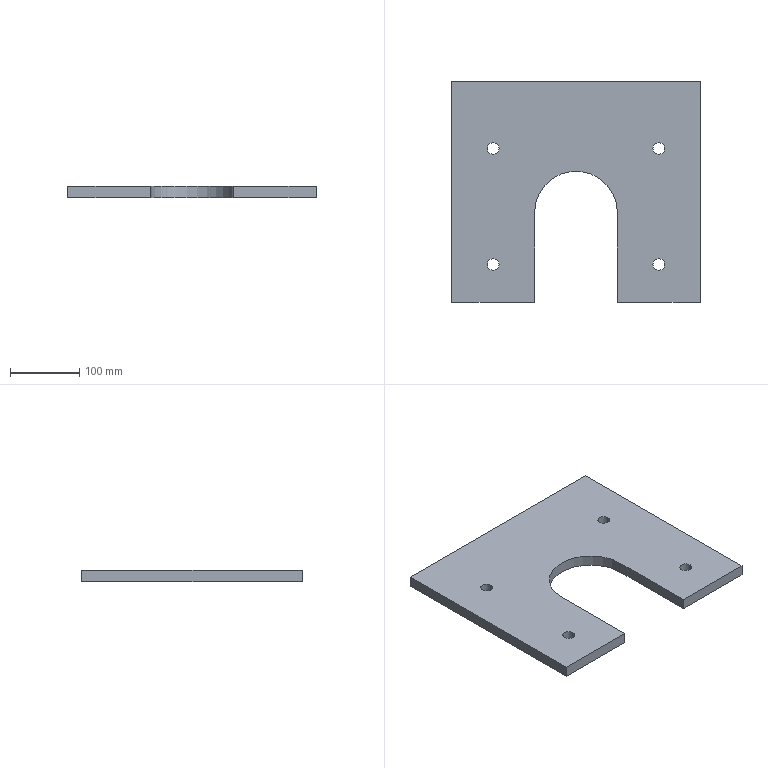Part | SolidWorks | features ICE 2, Extrusion 1, LPattern 1 | 1 solid | 18 faces | box 360 x 320 x 16 mm | volume 1488595 mm3 | cylinder 9 | plane 9 | commonest cylinder face diameters 17 x8 120 x1
STEP:
#1=CARTESIAN_POINT('',(111.5,-105.,-8.));
#2=VERTEX_POINT('',#1);
#3=CARTESIAN_POINT('',(128.5,-105.,-8.));
#4=VERTEX_POINT('',#3);
#5=CARTESIAN_POINT('',(120.,-105.,-8.));
#6=DIRECTION('',(0.,0.,1.));
#7=DIRECTION('',(1.,0.,0.));
#8=AXIS2_PLACEMENT_3D('',#5,#6,#7);
#9=CIRCLE('',#8,8.5);
#10=EDGE_CURVE('',#2,#4,#9,.T.);
#11=ORIENTED_EDGE('',*,*,#10,.F.);
#12=CARTESIAN_POINT('',(111.5,-105.,8.));
#13=VERTEX_POINT('',#12);
#14=CARTESIAN_POINT('',(111.5,-105.,-8.));
#15=DIRECTION('',(0.,0.,1.));
#16=VECTOR('',#15,1000.);
#17=LINE('',#14,#16);
#18=EDGE_CURVE('',#2,#13,#17,.T.);
#19=ORIENTED_EDGE('',*,*,#18,.T.);
#20=CARTESIAN_POINT('',(128.5,-105.,8.));
#21=VERTEX_POINT('',#20);
#22=CARTESIAN_POINT('',(120.,-105.,8.));
#23=DIRECTION('',(0.,0.,1.));
#24=DIRECTION('',(1.,0.,0.));
#25=AXIS2_PLACEMENT_3D('',#22,#23,#24);
#26=CIRCLE('',#25,8.5);
#27=EDGE_CURVE('',#13,#21,#26,.T.);
#28=ORIENTED_EDGE('',*,*,#27,.T.);
#29=CARTESIAN_POINT('',(128.5,-105.,-8.));
#30=DIRECTION('',(0.,0.,1.));
#31=VECTOR('',#30,1000.);
#32=LINE('',#29,#31);
#33=EDGE_CURVE('',#4,#21,#32,.T.);
#34=ORIENTED_EDGE('',*,*,#33,.F.);
#35=EDGE_LOOP('',(#11,#19,#28,#34));
#36=FACE_OUTER_BOUND('',#35,.T.);
#37=CARTESIAN_POINT('',(120.,-105.,-8.));
#38=DIRECTION('',(0.,0.,1.));
#39=DIRECTION('',(1.,0.,0.));
#40=AXIS2_PLACEMENT_3D('',#37,#38,#39);
#41=CYLINDRICAL_SURFACE('',#40,8.5);
#42=ADVANCED_FACE('',(#36),#41,.F.);
#43=CARTESIAN_POINT('',(-128.5,-105.,-8.));
#44=VERTEX_POINT('',#43);
#45=CARTESIAN_POINT('',(-111.5,-105.,-8.));
#46=VERTEX_POINT('',#45);
#47=CARTESIAN_POINT('',(-120.,-105.,-8.));
#48=DIRECTION('',(0.,0.,1.));
#49=DIRECTION('',(1.,0.,0.));
#50=AXIS2_PLACEMENT_3D('',#47,#48,#49);
#51=CIRCLE('',#50,8.5);
#52=EDGE_CURVE('',#44,#46,#51,.T.);
#53=ORIENTED_EDGE('',*,*,#52,.F.);
#54=CARTESIAN_POINT('',(-128.5,-105.,8.));
#55=VERTEX_POINT('',#54);
#56=CARTESIAN_POINT('',(-128.5,-105.,-8.));
#57=DIRECTION('',(0.,0.,1.));
#58=VECTOR('',#57,1000.);
#59=LINE('',#56,#58);
#60=EDGE_CURVE('',#44,#55,#59,.T.);
#61=ORIENTED_EDGE('',*,*,#60,.T.);
#62=CARTESIAN_POINT('',(-111.5,-105.,8.));
#63=VERTEX_POINT('',#62);
#64=CARTESIAN_POINT('',(-120.,-105.,8.));
#65=DIRECTION('',(0.,0.,1.));
#66=DIRECTION('',(1.,0.,0.));
#67=AXIS2_PLACEMENT_3D('',#64,#65,#66);
#68=CIRCLE('',#67,8.5);
#69=EDGE_CURVE('',#55,#63,#68,.T.);
#70=ORIENTED_EDGE('',*,*,#69,.T.);
#71=CARTESIAN_POINT('',(-111.5,-105.,-8.));
#72=DIRECTION('',(0.,0.,1.));
#73=VECTOR('',#72,1000.);
#74=LINE('',#71,#73);
#75=EDGE_CURVE('',#46,#63,#74,.T.);
#76=ORIENTED_EDGE('',*,*,#75,.F.);
#77=EDGE_LOOP('',(#53,#61,#70,#76));
#78=FACE_OUTER_BOUND('',#77,.T.);
#79=CARTESIAN_POINT('',(-120.,-105.,-8.));
#80=DIRECTION('',(0.,0.,1.));
#81=DIRECTION('',(1.,0.,0.));
#82=AXIS2_PLACEMENT_3D('',#79,#80,#81);
#83=CYLINDRICAL_SURFACE('',#82,8.5);
#84=ADVANCED_FACE('',(#78),#83,.F.);
#85=CARTESIAN_POINT('',(111.5,63.,-8.));
#86=VERTEX_POINT('',#85);
#87=CARTESIAN_POINT('',(128.5,63.,-8.));
#88=VERTEX_POINT('',#87);
#89=CARTESIAN_POINT('',(120.,63.,-8.));
#90=DIRECTION('',(0.,0.,1.));
#91=DIRECTION('',(1.,0.,0.));
#92=AXIS2_PLACEMENT_3D('',#89,#90,#91);
#93=CIRCLE('',#92,8.5);
#94=EDGE_CURVE('',#86,#88,#93,.T.);
#95=ORIENTED_EDGE('',*,*,#94,.F.);
#96=CARTESIAN_POINT('',(111.5,63.,8.));
#97=VERTEX_POINT('',#96);
#98=CARTESIAN_POINT('',(111.5,63.,-8.));
#99=DIRECTION('',(0.,0.,1.));
#100=VECTOR('',#99,1000.);
#101=LINE('',#98,#100);
#102=EDGE_CURVE('',#86,#97,#101,.T.);
#103=ORIENTED_EDGE('',*,*,#102,.T.);
#104=CARTESIAN_POINT('',(128.5,63.,8.));
#105=VERTEX_POINT('',#104);
#106=CARTESIAN_POINT('',(120.,63.,8.));
#107=DIRECTION('',(0.,0.,1.));
#108=DIRECTION('',(1.,0.,0.));
#109=AXIS2_PLACEMENT_3D('',#106,#107,#108);
#110=CIRCLE('',#109,8.5);
#111=EDGE_CURVE('',#97,#105,#110,.T.);
#112=ORIENTED_EDGE('',*,*,#111,.T.);
#113=CARTESIAN_POINT('',(128.5,63.,-8.));
#114=DIRECTION('',(0.,0.,1.));
#115=VECTOR('',#114,1000.);
#116=LINE('',#113,#115);
#117=EDGE_CURVE('',#88,#105,#116,.T.);
#118=ORIENTED_EDGE('',*,*,#117,.F.);
#119=EDGE_LOOP('',(#95,#103,#112,#118));
#120=FACE_OUTER_BOUND('',#119,.T.);
#121=CARTESIAN_POINT('',(120.,63.,-8.));
#122=DIRECTION('',(0.,0.,1.));
#123=DIRECTION('',(1.,0.,0.));
#124=AXIS2_PLACEMENT_3D('',#121,#122,#123);
#125=CYLINDRICAL_SURFACE('',#124,8.5);
#126=ADVANCED_FACE('',(#120),#125,.F.);
#127=CARTESIAN_POINT('',(-128.5,63.,-8.));
#128=VERTEX_POINT('',#127);
#129=CARTESIAN_POINT('',(-111.5,63.,-8.));
#130=VERTEX_POINT('',#129);
#131=CARTESIAN_POINT('',(-120.,63.,-8.));
#132=DIRECTION('',(0.,0.,1.));
#133=DIRECTION('',(1.,0.,0.));
#134=AXIS2_PLACEMENT_3D('',#131,#132,#133);
#135=CIRCLE('',#134,8.5);
#136=EDGE_CURVE('',#128,#130,#135,.T.);
#137=ORIENTED_EDGE('',*,*,#136,.F.);
#138=CARTESIAN_POINT('',(-128.5,63.,8.));
#139=VERTEX_POINT('',#138);
#140=CARTESIAN_POINT('',(-128.5,63.,-8.));
#141=DIRECTION('',(0.,0.,1.));
#142=VECTOR('',#141,1000.);
#143=LINE('',#140,#142);
#144=EDGE_CURVE('',#128,#139,#143,.T.);
#145=ORIENTED_EDGE('',*,*,#144,.T.);
#146=CARTESIAN_POINT('',(-111.5,63.,8.));
#147=VERTEX_POINT('',#146);
#148=CARTESIAN_POINT('',(-120.,63.,8.));
#149=DIRECTION('',(0.,0.,1.));
#150=DIRECTION('',(1.,0.,0.));
#151=AXIS2_PLACEMENT_3D('',#148,#149,#150);
#152=CIRCLE('',#151,8.5);
#153=EDGE_CURVE('',#139,#147,#152,.T.);
#154=ORIENTED_EDGE('',*,*,#153,.T.);
#155=CARTESIAN_POINT('',(-111.5,63.,-8.));
#156=DIRECTION('',(0.,0.,1.));
#157=VECTOR('',#156,1000.);
#158=LINE('',#155,#157);
#159=EDGE_CURVE('',#130,#147,#158,.T.);
#160=ORIENTED_EDGE('',*,*,#159,.F.);
#161=EDGE_LOOP('',(#137,#145,#154,#160));
#162=FACE_OUTER_BOUND('',#161,.T.);
#163=CARTESIAN_POINT('',(-120.,63.,-8.));
#164=DIRECTION('',(0.,0.,1.));
#165=DIRECTION('',(1.,0.,0.));
#166=AXIS2_PLACEMENT_3D('',#163,#164,#165);
#167=CYLINDRICAL_SURFACE('',#166,8.5);
#168=ADVANCED_FACE('',(#162),#167,.F.);
#169=CARTESIAN_POINT('',(-180.,-160.,-8.));
#170=VERTEX_POINT('',#169);
#171=CARTESIAN_POINT('',(-60.,-160.,-8.));
#172=VERTEX_POINT('',#171);
#173=CARTESIAN_POINT('',(180.,-160.,-8.));
#174=DIRECTION('',(1.,0.,0.));
#175=VECTOR('',#174,1000.);
#176=LINE('',#173,#175);
#177=EDGE_CURVE('',#170,#172,#176,.T.);
#178=ORIENTED_EDGE('',*,*,#177,.T.);
#179=CARTESIAN_POINT('',(-60.,-160.,8.));
#180=VERTEX_POINT('',#179);
#181=CARTESIAN_POINT('',(-60.,-160.,-8.));
#182=DIRECTION('',(0.,0.,1.));
#183=VECTOR('',#182,1000.);
#184=LINE('',#181,#183);
#185=EDGE_CURVE('',#172,#180,#184,.T.);
#186=ORIENTED_EDGE('',*,*,#185,.T.);
#187=CARTESIAN_POINT('',(-180.,-160.,8.));
#188=VERTEX_POINT('',#187);
#189=CARTESIAN_POINT('',(180.,-160.,8.));
#190=DIRECTION('',(1.,0.,0.));
#191=VECTOR('',#190,1000.);
#192=LINE('',#189,#191);
#193=EDGE_CURVE('',#188,#180,#192,.T.);
#194=ORIENTED_EDGE('',*,*,#193,.F.);
#195=CARTESIAN_POINT('',(-180.,-160.,8.));
#196=DIRECTION('',(0.,0.,-1.));
#197=VECTOR('',#196,1000.);
#198=LINE('',#195,#197);
#199=EDGE_CURVE('',#188,#170,#198,.T.);
#200=ORIENTED_EDGE('',*,*,#199,.T.);
#201=EDGE_LOOP('',(#178,#186,#194,#200));
#202=FACE_OUTER_BOUND('',#201,.T.);
#203=CARTESIAN_POINT('',(180.,-160.,8.));
#204=DIRECTION('',(0.,1.,0.));
#205=DIRECTION('',(0.,0.,1.));
#206=AXIS2_PLACEMENT_3D('',#203,#204,#205);
#207=PLANE('',#206);
#208=ADVANCED_FACE('',(#202),#207,.F.);
#209=CARTESIAN_POINT('',(-180.,160.,-8.));
#210=VERTEX_POINT('',#209);
#211=CARTESIAN_POINT('',(-180.,-160.,-8.));
#212=DIRECTION('',(0.,-1.,0.));
#213=VECTOR('',#212,1000.);
#214=LINE('',#211,#213);
#215=EDGE_CURVE('',#210,#170,#214,.T.);
#216=ORIENTED_EDGE('',*,*,#215,.T.);
#217=ORIENTED_EDGE('',*,*,#199,.F.);
#218=CARTESIAN_POINT('',(-180.,160.,8.));
#219=VERTEX_POINT('',#218);
#220=CARTESIAN_POINT('',(-180.,-160.,8.));
#221=DIRECTION('',(0.,-1.,0.));
#222=VECTOR('',#221,1000.);
#223=LINE('',#220,#222);
#224=EDGE_CURVE('',#219,#188,#223,.T.);
#225=ORIENTED_EDGE('',*,*,#224,.F.);
#226=CARTESIAN_POINT('',(-180.,160.,8.));
#227=DIRECTION('',(0.,0.,-1.));
#228=VECTOR('',#227,1000.);
#229=LINE('',#226,#228);
#230=EDGE_CURVE('',#219,#210,#229,.T.);
#231=ORIENTED_EDGE('',*,*,#230,.T.);
#232=EDGE_LOOP('',(#216,#217,#225,#231));
#233=FACE_OUTER_BOUND('',#232,.T.);
#234=CARTESIAN_POINT('',(-180.,-160.,8.));
#235=DIRECTION('',(1.,0.,0.));
#236=DIRECTION('',(0.,1.,0.));
#237=AXIS2_PLACEMENT_3D('',#234,#235,#236);
#238=PLANE('',#237);
#239=ADVANCED_FACE('',(#233),#238,.F.);
#240=CARTESIAN_POINT('',(60.,-160.,8.));
#241=VERTEX_POINT('',#240);
#242=CARTESIAN_POINT('',(180.,-160.,8.));
#243=VERTEX_POINT('',#242);
#244=CARTESIAN_POINT('',(180.,-160.,8.));
#245=DIRECTION('',(1.,0.,0.));
#246=VECTOR('',#245,1000.);
#247=LINE('',#244,#246);
#248=EDGE_CURVE('',#241,#243,#247,.T.);
#249=ORIENTED_EDGE('',*,*,#248,.F.);
#250=CARTESIAN_POINT('',(60.,-160.,-8.));
#251=VERTEX_POINT('',#250);
#252=CARTESIAN_POINT('',(60.,-160.,-8.));
#253=DIRECTION('',(0.,0.,1.));
#254=VECTOR('',#253,1000.);
#255=LINE('',#252,#254);
#256=EDGE_CURVE('',#251,#241,#255,.T.);
#257=ORIENTED_EDGE('',*,*,#256,.F.);
#258=CARTESIAN_POINT('',(180.,-160.,-8.));
#259=VERTEX_POINT('',#258);
#260=CARTESIAN_POINT('',(180.,-160.,-8.));
#261=DIRECTION('',(1.,0.,0.));
#262=VECTOR('',#261,1000.);
#263=LINE('',#260,#262);
#264=EDGE_CURVE('',#251,#259,#263,.T.);
#265=ORIENTED_EDGE('',*,*,#264,.T.);
#266=CARTESIAN_POINT('',(180.,-160.,8.));
#267=DIRECTION('',(0.,0.,-1.));
#268=VECTOR('',#267,1000.);
#269=LINE('',#266,#268);
#270=EDGE_CURVE('',#243,#259,#269,.T.);
#271=ORIENTED_EDGE('',*,*,#270,.F.);
#272=EDGE_LOOP('',(#249,#257,#265,#271));
#273=FACE_OUTER_BOUND('',#272,.T.);
#274=CARTESIAN_POINT('',(180.,-160.,8.));
#275=DIRECTION('',(0.,1.,0.));
#276=DIRECTION('',(0.,0.,1.));
#277=AXIS2_PLACEMENT_3D('',#274,#275,#276);
#278=PLANE('',#277);
#279=ADVANCED_FACE('',(#273),#278,.F.);
#280=CARTESIAN_POINT('',(180.,160.,-8.));
#281=VERTEX_POINT('',#280);
#282=CARTESIAN_POINT('',(180.,160.,-8.));
#283=DIRECTION('',(0.,1.,0.));
#284=VECTOR('',#283,1000.);
#285=LINE('',#282,#284);
#286=EDGE_CURVE('',#259,#281,#285,.T.);
#287=ORIENTED_EDGE('',*,*,#286,.T.);
#288=CARTESIAN_POINT('',(180.,160.,8.));
#289=VERTEX_POINT('',#288);
#290=CARTESIAN_POINT('',(180.,160.,8.));
#291=DIRECTION('',(0.,0.,-1.));
#292=VECTOR('',#291,1000.);
#293=LINE('',#290,#292);
#294=EDGE_CURVE('',#289,#281,#293,.T.);
#295=ORIENTED_EDGE('',*,*,#294,.F.);
#296=CARTESIAN_POINT('',(180.,160.,8.));
#297=DIRECTION('',(0.,1.,0.));
#298=VECTOR('',#297,1000.);
#299=LINE('',#296,#298);
#300=EDGE_CURVE('',#243,#289,#299,.T.);
#301=ORIENTED_EDGE('',*,*,#300,.F.);
#302=ORIENTED_EDGE('',*,*,#270,.T.);
#303=EDGE_LOOP('',(#287,#295,#301,#302));
#304=FACE_OUTER_BOUND('',#303,.T.);
#305=CARTESIAN_POINT('',(180.,160.,8.));
#306=DIRECTION('',(-1.,0.,0.));
#307=DIRECTION('',(0.,-1.,0.));
#308=AXIS2_PLACEMENT_3D('',#305,#306,#307);
#309=PLANE('',#308);
#310=ADVANCED_FACE('',(#304),#309,.F.);
#311=CARTESIAN_POINT('',(-180.,160.,-8.));
#312=DIRECTION('',(-1.,0.,0.));
#313=VECTOR('',#312,1000.);
#314=LINE('',#311,#313);
#315=EDGE_CURVE('',#281,#210,#314,.T.);
#316=ORIENTED_EDGE('',*,*,#315,.T.);
#317=ORIENTED_EDGE('',*,*,#230,.F.);
#318=CARTESIAN_POINT('',(-180.,160.,8.));
#319=DIRECTION('',(-1.,0.,0.));
#320=VECTOR('',#319,1000.);
#321=LINE('',#318,#320);
#322=EDGE_CURVE('',#289,#219,#321,.T.);
#323=ORIENTED_EDGE('',*,*,#322,.F.);
#324=ORIENTED_EDGE('',*,*,#294,.T.);
#325=EDGE_LOOP('',(#316,#317,#323,#324));
#326=FACE_OUTER_BOUND('',#325,.T.);
#327=CARTESIAN_POINT('',(-180.,160.,8.));
#328=DIRECTION('',(0.,-1.,0.));
#329=DIRECTION('',(0.,0.,-1.));
#330=AXIS2_PLACEMENT_3D('',#327,#328,#329);
#331=PLANE('',#330);
#332=ADVANCED_FACE('',(#326),#331,.F.);
#333=CARTESIAN_POINT('',(120.,63.,8.));
#334=DIRECTION('',(0.,0.,1.));
#335=DIRECTION('',(1.,0.,0.));
#336=AXIS2_PLACEMENT_3D('',#333,#334,#335);
#337=CIRCLE('',#336,8.5);
#338=EDGE_CURVE('',#105,#97,#337,.T.);
#339=ORIENTED_EDGE('',*,*,#338,.F.);
#340=ORIENTED_EDGE('',*,*,#111,.F.);
#341=EDGE_LOOP('',(#339,#340));
#342=FACE_BOUND('',#341,.T.);
#343=CARTESIAN_POINT('',(-120.,63.,8.));
#344=DIRECTION('',(0.,0.,1.));
#345=DIRECTION('',(1.,0.,0.));
#346=AXIS2_PLACEMENT_3D('',#343,#344,#345);
#347=CIRCLE('',#346,8.5);
#348=EDGE_CURVE('',#147,#139,#347,.T.);
#349=ORIENTED_EDGE('',*,*,#348,.F.);
#350=ORIENTED_EDGE('',*,*,#153,.F.);
#351=EDGE_LOOP('',(#349,#350));
#352=FACE_BOUND('',#351,.T.);
#353=ORIENTED_EDGE('',*,*,#193,.T.);
#354=CARTESIAN_POINT('',(-60.,-30.,8.));
#355=VERTEX_POINT('',#354);
#356=CARTESIAN_POINT('',(-60.,-160.,8.));
#357=DIRECTION('',(0.,-1.,0.));
#358=VECTOR('',#357,1000.);
#359=LINE('',#356,#358);
#360=EDGE_CURVE('',#355,#180,#359,.T.);
#361=ORIENTED_EDGE('',*,*,#360,.F.);
#362=CARTESIAN_POINT('',(60.,-30.,8.));
#363=VERTEX_POINT('',#362);
#364=CARTESIAN_POINT('',(0.,-30.,8.));
#365=DIRECTION('',(0.,0.,1.));
#366=DIRECTION('',(-1.,0.,0.));
#367=AXIS2_PLACEMENT_3D('',#364,#365,#366);
#368=CIRCLE('',#367,60.);
#369=EDGE_CURVE('',#363,#355,#368,.T.);
#370=ORIENTED_EDGE('',*,*,#369,.F.);
#371=CARTESIAN_POINT('',(60.,-160.,8.));
#372=DIRECTION('',(0.,1.,0.));
#373=VECTOR('',#372,1000.);
#374=LINE('',#371,#373);
#375=EDGE_CURVE('',#241,#363,#374,.T.);
#376=ORIENTED_EDGE('',*,*,#375,.F.);
#377=ORIENTED_EDGE('',*,*,#248,.T.);
#378=ORIENTED_EDGE('',*,*,#300,.T.);
#379=ORIENTED_EDGE('',*,*,#322,.T.);
#380=ORIENTED_EDGE('',*,*,#224,.T.);
#381=EDGE_LOOP('',(#353,#361,#370,#376,#377,#378,#379,#380));
#382=FACE_OUTER_BOUND('',#381,.T.);
#383=CARTESIAN_POINT('',(-120.,-105.,8.));
#384=DIRECTION('',(0.,0.,1.));
#385=DIRECTION('',(1.,0.,0.));
#386=AXIS2_PLACEMENT_3D('',#383,#384,#385);
#387=CIRCLE('',#386,8.5);
#388=EDGE_CURVE('',#63,#55,#387,.T.);
#389=ORIENTED_EDGE('',*,*,#388,.F.);
#390=ORIENTED_EDGE('',*,*,#69,.F.);
#391=EDGE_LOOP('',(#389,#390));
#392=FACE_BOUND('',#391,.T.);
#393=CARTESIAN_POINT('',(120.,-105.,8.));
#394=DIRECTION('',(0.,0.,1.));
#395=DIRECTION('',(1.,0.,0.));
#396=AXIS2_PLACEMENT_3D('',#393,#394,#395);
#397=CIRCLE('',#396,8.5);
#398=EDGE_CURVE('',#21,#13,#397,.T.);
#399=ORIENTED_EDGE('',*,*,#398,.F.);
#400=ORIENTED_EDGE('',*,*,#27,.F.);
#401=EDGE_LOOP('',(#399,#400));
#402=FACE_BOUND('',#401,.T.);
#403=CARTESIAN_POINT('',(-180.,160.,8.));
#404=DIRECTION('',(0.,0.,-1.));
#405=DIRECTION('',(-1.,0.,0.));
#406=AXIS2_PLACEMENT_3D('',#403,#404,#405);
#407=PLANE('',#406);
#408=ADVANCED_FACE('',(#342,#352,#382,#392,#402),#407,.F.);
#409=CARTESIAN_POINT('',(120.,63.,-8.));
#410=DIRECTION('',(0.,0.,1.));
#411=DIRECTION('',(1.,0.,0.));
#412=AXIS2_PLACEMENT_3D('',#409,#410,#411);
#413=CIRCLE('',#412,8.5);
#414=EDGE_CURVE('',#88,#86,#413,.T.);
#415=ORIENTED_EDGE('',*,*,#414,.T.);
#416=ORIENTED_EDGE('',*,*,#94,.T.);
#417=EDGE_LOOP('',(#415,#416));
#418=FACE_BOUND('',#417,.T.);
#419=CARTESIAN_POINT('',(-120.,63.,-8.));
#420=DIRECTION('',(0.,0.,1.));
#421=DIRECTION('',(1.,0.,0.));
#422=AXIS2_PLACEMENT_3D('',#419,#420,#421);
#423=CIRCLE('',#422,8.5);
#424=EDGE_CURVE('',#130,#128,#423,.T.);
#425=ORIENTED_EDGE('',*,*,#424,.T.);
#426=ORIENTED_EDGE('',*,*,#136,.T.);
#427=EDGE_LOOP('',(#425,#426));
#428=FACE_BOUND('',#427,.T.);
#429=CARTESIAN_POINT('',(-60.,-30.,-8.));
#430=VERTEX_POINT('',#429);
#431=CARTESIAN_POINT('',(-60.,-160.,-8.));
#432=DIRECTION('',(0.,-1.,0.));
#433=VECTOR('',#432,1000.);
#434=LINE('',#431,#433);
#435=EDGE_CURVE('',#430,#172,#434,.T.);
#436=ORIENTED_EDGE('',*,*,#435,.T.);
#437=ORIENTED_EDGE('',*,*,#177,.F.);
#438=ORIENTED_EDGE('',*,*,#215,.F.);
#439=ORIENTED_EDGE('',*,*,#315,.F.);
#440=ORIENTED_EDGE('',*,*,#286,.F.);
#441=ORIENTED_EDGE('',*,*,#264,.F.);
#442=CARTESIAN_POINT('',(60.,-30.,-8.));
#443=VERTEX_POINT('',#442);
#444=CARTESIAN_POINT('',(60.,-160.,-8.));
#445=DIRECTION('',(0.,1.,0.));
#446=VECTOR('',#445,1000.);
#447=LINE('',#444,#446);
#448=EDGE_CURVE('',#251,#443,#447,.T.);
#449=ORIENTED_EDGE('',*,*,#448,.T.);
#450=CARTESIAN_POINT('',(0.,-30.,-8.));
#451=DIRECTION('',(0.,0.,1.));
#452=DIRECTION('',(-1.,0.,0.));
#453=AXIS2_PLACEMENT_3D('',#450,#451,#452);
#454=CIRCLE('',#453,60.);
#455=EDGE_CURVE('',#443,#430,#454,.T.);
#456=ORIENTED_EDGE('',*,*,#455,.T.);
#457=EDGE_LOOP('',(#436,#437,#438,#439,#440,#441,#449,#456));
#458=FACE_OUTER_BOUND('',#457,.T.);
#459=CARTESIAN_POINT('',(-120.,-105.,-8.));
#460=DIRECTION('',(0.,0.,1.));
#461=DIRECTION('',(1.,0.,0.));
#462=AXIS2_PLACEMENT_3D('',#459,#460,#461);
#463=CIRCLE('',#462,8.5);
#464=EDGE_CURVE('',#46,#44,#463,.T.);
#465=ORIENTED_EDGE('',*,*,#464,.T.);
#466=ORIENTED_EDGE('',*,*,#52,.T.);
#467=EDGE_LOOP('',(#465,#466));
#468=FACE_BOUND('',#467,.T.);
#469=CARTESIAN_POINT('',(120.,-105.,-8.));
#470=DIRECTION('',(0.,0.,1.));
#471=DIRECTION('',(1.,0.,0.));
#472=AXIS2_PLACEMENT_3D('',#469,#470,#471);
#473=CIRCLE('',#472,8.5);
#474=EDGE_CURVE('',#4,#2,#473,.T.);
#475=ORIENTED_EDGE('',*,*,#474,.T.);
#476=ORIENTED_EDGE('',*,*,#10,.T.);
#477=EDGE_LOOP('',(#475,#476));
#478=FACE_BOUND('',#477,.T.);
#479=CARTESIAN_POINT('',(-180.,160.,-8.));
#480=DIRECTION('',(0.,0.,-1.));
#481=DIRECTION('',(-1.,0.,0.));
#482=AXIS2_PLACEMENT_3D('',#479,#480,#481);
#483=PLANE('',#482);
#484=ADVANCED_FACE('',(#418,#428,#458,#468,#478),#483,.T.);
#485=ORIENTED_EDGE('',*,*,#360,.T.);
#486=ORIENTED_EDGE('',*,*,#185,.F.);
#487=ORIENTED_EDGE('',*,*,#435,.F.);
#488=CARTESIAN_POINT('',(-60.,-30.,-8.));
#489=DIRECTION('',(0.,0.,1.));
#490=VECTOR('',#489,1000.);
#491=LINE('',#488,#490);
#492=EDGE_CURVE('',#430,#355,#491,.T.);
#493=ORIENTED_EDGE('',*,*,#492,.T.);
#494=EDGE_LOOP('',(#485,#486,#487,#493));
#495=FACE_OUTER_BOUND('',#494,.T.);
#496=CARTESIAN_POINT('',(-60.,-160.,-8.));
#497=DIRECTION('',(-1.,0.,0.));
#498=DIRECTION('',(0.,-1.,0.));
#499=AXIS2_PLACEMENT_3D('',#496,#497,#498);
#500=PLANE('',#499);
#501=ADVANCED_FACE('',(#495),#500,.F.);
#502=ORIENTED_EDGE('',*,*,#369,.T.);
#503=ORIENTED_EDGE('',*,*,#492,.F.);
#504=ORIENTED_EDGE('',*,*,#455,.F.);
#505=CARTESIAN_POINT('',(60.,-30.,-8.));
#506=DIRECTION('',(0.,0.,1.));
#507=VECTOR('',#506,1000.);
#508=LINE('',#505,#507);
#509=EDGE_CURVE('',#443,#363,#508,.T.);
#510=ORIENTED_EDGE('',*,*,#509,.T.);
#511=EDGE_LOOP('',(#502,#503,#504,#510));
#512=FACE_OUTER_BOUND('',#511,.T.);
#513=CARTESIAN_POINT('',(0.,-30.,-8.));
#514=DIRECTION('',(0.,0.,1.));
#515=DIRECTION('',(1.,0.,0.));
#516=AXIS2_PLACEMENT_3D('',#513,#514,#515);
#517=CYLINDRICAL_SURFACE('',#516,60.);
#518=ADVANCED_FACE('',(#512),#517,.F.);
#519=ORIENTED_EDGE('',*,*,#375,.T.);
#520=ORIENTED_EDGE('',*,*,#509,.F.);
#521=ORIENTED_EDGE('',*,*,#448,.F.);
#522=ORIENTED_EDGE('',*,*,#256,.T.);
#523=EDGE_LOOP('',(#519,#520,#521,#522));
#524=FACE_OUTER_BOUND('',#523,.T.);
#525=CARTESIAN_POINT('',(60.,-160.,-8.));
#526=DIRECTION('',(1.,0.,0.));
#527=DIRECTION('',(0.,0.,-1.));
#528=AXIS2_PLACEMENT_3D('',#525,#526,#527);
#529=PLANE('',#528);
#530=ADVANCED_FACE('',(#524),#529,.F.);
#531=ORIENTED_EDGE('',*,*,#144,.F.);
#532=ORIENTED_EDGE('',*,*,#424,.F.);
#533=ORIENTED_EDGE('',*,*,#159,.T.);
#534=ORIENTED_EDGE('',*,*,#348,.T.);
#535=EDGE_LOOP('',(#531,#532,#533,#534));
#536=FACE_OUTER_BOUND('',#535,.T.);
#537=CARTESIAN_POINT('',(-120.,63.,-8.));
#538=DIRECTION('',(0.,0.,1.));
#539=DIRECTION('',(1.,0.,0.));
#540=AXIS2_PLACEMENT_3D('',#537,#538,#539);
#541=CYLINDRICAL_SURFACE('',#540,8.5);
#542=ADVANCED_FACE('',(#536),#541,.F.);
#543=ORIENTED_EDGE('',*,*,#102,.F.);
#544=ORIENTED_EDGE('',*,*,#414,.F.);
#545=ORIENTED_EDGE('',*,*,#117,.T.);
#546=ORIENTED_EDGE('',*,*,#338,.T.);
#547=EDGE_LOOP('',(#543,#544,#545,#546));
#548=FACE_OUTER_BOUND('',#547,.T.);
#549=CARTESIAN_POINT('',(120.,63.,-8.));
#550=DIRECTION('',(0.,0.,1.));
#551=DIRECTION('',(1.,0.,0.));
#552=AXIS2_PLACEMENT_3D('',#549,#550,#551);
#553=CYLINDRICAL_SURFACE('',#552,8.5);
#554=ADVANCED_FACE('',(#548),#553,.F.);
#555=ORIENTED_EDGE('',*,*,#60,.F.);
#556=ORIENTED_EDGE('',*,*,#464,.F.);
#557=ORIENTED_EDGE('',*,*,#75,.T.);
#558=ORIENTED_EDGE('',*,*,#388,.T.);
#559=EDGE_LOOP('',(#555,#556,#557,#558));
#560=FACE_OUTER_BOUND('',#559,.T.);
#561=CARTESIAN_POINT('',(-120.,-105.,-8.));
#562=DIRECTION('',(0.,0.,1.));
#563=DIRECTION('',(1.,0.,0.));
#564=AXIS2_PLACEMENT_3D('',#561,#562,#563);
#565=CYLINDRICAL_SURFACE('',#564,8.5);
#566=ADVANCED_FACE('',(#560),#565,.F.);
#567=ORIENTED_EDGE('',*,*,#18,.F.);
#568=ORIENTED_EDGE('',*,*,#474,.F.);
#569=ORIENTED_EDGE('',*,*,#33,.T.);
#570=ORIENTED_EDGE('',*,*,#398,.T.);
#571=EDGE_LOOP('',(#567,#568,#569,#570));
#572=FACE_OUTER_BOUND('',#571,.T.);
#573=CARTESIAN_POINT('',(120.,-105.,-8.));
#574=DIRECTION('',(0.,0.,1.));
#575=DIRECTION('',(1.,0.,0.));
#576=AXIS2_PLACEMENT_3D('',#573,#574,#575);
#577=CYLINDRICAL_SURFACE('',#576,8.5);
#578=ADVANCED_FACE('',(#572),#577,.F.);
#579=CLOSED_SHELL('',(#42,#84,#126,#168,#208,#239,#279,#310,#332,#408,#484,#501,#518,#530,#542,#554,#566,#578));
#580=MANIFOLD_SOLID_BREP('',#579);
#581=CARTESIAN_POINT('',(0.,0.,0.));
#582=DIRECTION('',(0.,0.,1.));
#583=DIRECTION('',(1.,0.,0.));
#584=AXIS2_PLACEMENT_3D('',#581,#582,#583);
#585=(LENGTH_UNIT()NAMED_UNIT(*)SI_UNIT(.MILLI.,.METRE.));
#586=UNCERTAINTY_MEASURE_WITH_UNIT(LENGTH_MEASURE(0.00001),#585,'','');
#587=(NAMED_UNIT(*)PLANE_ANGLE_UNIT()SI_UNIT($,.RADIAN.));
#588=(NAMED_UNIT(*)SI_UNIT($,.STERADIAN.)SOLID_ANGLE_UNIT());
#589=(GEOMETRIC_REPRESENTATION_CONTEXT(3)GLOBAL_UNCERTAINTY_ASSIGNED_CONTEXT((#586))GLOBAL_UNIT_ASSIGNED_CONTEXT((#585,#587,#588))REPRESENTATION_CONTEXT('',''));
#590=ADVANCED_BREP_SHAPE_REPRESENTATION('',(#580,#584),#589);